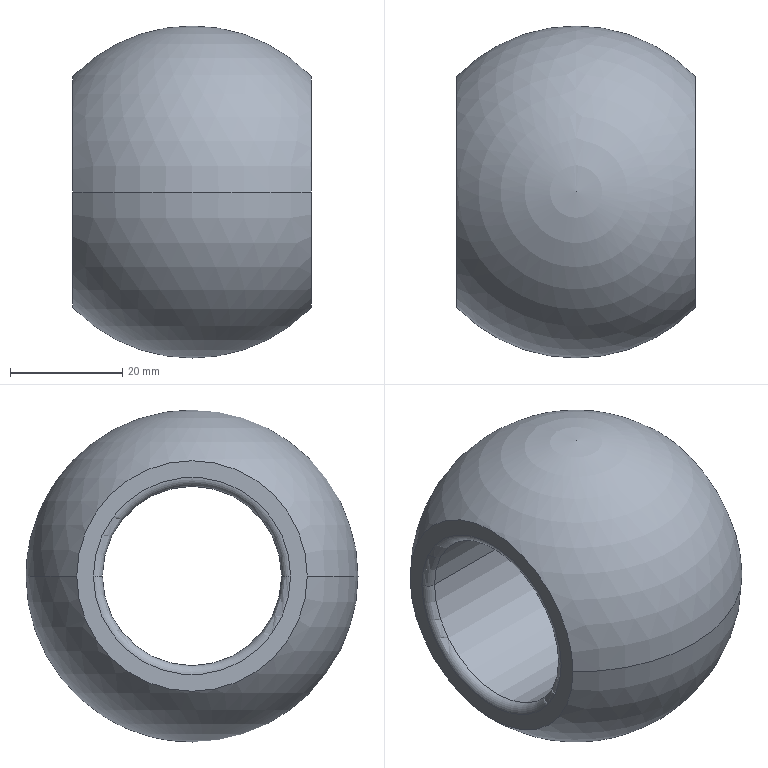Part | STEP file | Large rod end bearing | 1 solid | 10 faces | box 42.667 x 59.28 x 59.28 mm | volume 62997 mm3 | torus 4 | sphere 2 | cylinder 2 | plane 2 | commonest cylinder face diameters 32 x2
STEP:
#1=CARTESIAN_POINT('',(21.333,20.577,261.));
#2=VERTEX_POINT('',#1);
#3=CARTESIAN_POINT('',(21.333,-20.577,261.));
#4=VERTEX_POINT('',#3);
#5=CARTESIAN_POINT('',(21.333,0.,261.));
#6=DIRECTION('',(-1.,0.,0.));
#7=DIRECTION('',(0.,-1.,0.));
#8=AXIS2_PLACEMENT_3D('',#5,#6,#7);
#9=CIRCLE('',#8,20.577);
#10=EDGE_CURVE('',#2,#4,#9,.T.);
#11=ORIENTED_EDGE('',*,*,#10,.T.);
#12=CARTESIAN_POINT('',(-21.333,-20.577,261.));
#13=VERTEX_POINT('',#12);
#14=CARTESIAN_POINT('',(0.,0.,261.));
#15=DIRECTION('',(0.,0.,-1.));
#16=DIRECTION('',(0.,1.,0.));
#17=AXIS2_PLACEMENT_3D('',#14,#15,#16);
#18=CIRCLE('',#17,29.64);
#19=EDGE_CURVE('',#4,#13,#18,.T.);
#20=ORIENTED_EDGE('',*,*,#19,.T.);
#21=CARTESIAN_POINT('',(-21.333,20.577,261.));
#22=VERTEX_POINT('',#21);
#23=CARTESIAN_POINT('',(-21.333,0.,261.));
#24=DIRECTION('',(-1.,0.,0.));
#25=DIRECTION('',(0.,-1.,0.));
#26=AXIS2_PLACEMENT_3D('',#23,#24,#25);
#27=CIRCLE('',#26,20.577);
#28=EDGE_CURVE('',#22,#13,#27,.T.);
#29=ORIENTED_EDGE('',*,*,#28,.F.);
#30=CARTESIAN_POINT('',(0.,0.,261.));
#31=DIRECTION('',(0.,0.,1.));
#32=DIRECTION('',(1.,0.,0.));
#33=AXIS2_PLACEMENT_3D('',#30,#31,#32);
#34=CIRCLE('',#33,29.64);
#35=EDGE_CURVE('',#2,#22,#34,.T.);
#36=ORIENTED_EDGE('',*,*,#35,.F.);
#37=EDGE_LOOP('',(#11,#20,#29,#36));
#38=FACE_OUTER_BOUND('',#37,.T.);
#39=CARTESIAN_POINT('',(0.,0.,261.));
#40=DIRECTION('',(0.,0.,-1.));
#41=DIRECTION('',(0.,1.,0.));
#42=AXIS2_PLACEMENT_3D('',#39,#40,#41);
#43=SPHERICAL_SURFACE('',#42,29.64);
#44=ADVANCED_FACE('',(#38),#43,.T.);
#45=CARTESIAN_POINT('',(-21.333,-17.6,261.));
#46=VERTEX_POINT('',#45);
#47=CARTESIAN_POINT('',(-21.333,17.6,261.));
#48=VERTEX_POINT('',#47);
#49=CARTESIAN_POINT('',(-21.333,0.,261.));
#50=DIRECTION('',(-1.,0.,0.));
#51=DIRECTION('',(0.,-1.,0.));
#52=AXIS2_PLACEMENT_3D('',#49,#50,#51);
#53=CIRCLE('',#52,17.6);
#54=EDGE_CURVE('',#46,#48,#53,.T.);
#55=ORIENTED_EDGE('',*,*,#54,.T.);
#56=CARTESIAN_POINT('',(-19.733,16.,261.));
#57=VERTEX_POINT('',#56);
#58=CARTESIAN_POINT('',(-19.733,17.6,261.));
#59=DIRECTION('',(0.,0.,1.));
#60=DIRECTION('',(0.,-1.,0.));
#61=AXIS2_PLACEMENT_3D('',#58,#59,#60);
#62=CIRCLE('',#61,1.6);
#63=EDGE_CURVE('',#48,#57,#62,.T.);
#64=ORIENTED_EDGE('',*,*,#63,.T.);
#65=CARTESIAN_POINT('',(-19.733,-16.,261.));
#66=VERTEX_POINT('',#65);
#67=CARTESIAN_POINT('',(-19.733,0.,261.));
#68=DIRECTION('',(-1.,0.,0.));
#69=DIRECTION('',(0.,-1.,0.));
#70=AXIS2_PLACEMENT_3D('',#67,#68,#69);
#71=CIRCLE('',#70,16.);
#72=EDGE_CURVE('',#66,#57,#71,.T.);
#73=ORIENTED_EDGE('',*,*,#72,.F.);
#74=CARTESIAN_POINT('',(-19.733,-17.6,261.));
#75=DIRECTION('',(0.,0.,-1.));
#76=DIRECTION('',(-1.,0.,0.));
#77=AXIS2_PLACEMENT_3D('',#74,#75,#76);
#78=CIRCLE('',#77,1.6);
#79=EDGE_CURVE('',#46,#66,#78,.T.);
#80=ORIENTED_EDGE('',*,*,#79,.F.);
#81=EDGE_LOOP('',(#55,#64,#73,#80));
#82=FACE_OUTER_BOUND('',#81,.T.);
#83=CARTESIAN_POINT('',(-19.733,0.,261.));
#84=DIRECTION('',(-1.,0.,0.));
#85=DIRECTION('',(0.,-1.,0.));
#86=AXIS2_PLACEMENT_3D('',#83,#84,#85);
#87=TOROIDAL_SURFACE('',#86,17.6,1.6);
#88=ADVANCED_FACE('',(#82),#87,.T.);
#89=CARTESIAN_POINT('',(19.733,16.,261.));
#90=VERTEX_POINT('',#89);
#91=CARTESIAN_POINT('',(19.733,-16.,261.));
#92=VERTEX_POINT('',#91);
#93=CARTESIAN_POINT('',(19.733,0.,261.));
#94=DIRECTION('',(-1.,0.,0.));
#95=DIRECTION('',(0.,-1.,0.));
#96=AXIS2_PLACEMENT_3D('',#93,#94,#95);
#97=CIRCLE('',#96,16.);
#98=EDGE_CURVE('',#90,#92,#97,.T.);
#99=ORIENTED_EDGE('',*,*,#98,.F.);
#100=CARTESIAN_POINT('',(21.333,16.,261.));
#101=DIRECTION('',(-1.,0.,0.));
#102=VECTOR('',#101,1000.);
#103=LINE('',#100,#102);
#104=EDGE_CURVE('',#90,#57,#103,.T.);
#105=ORIENTED_EDGE('',*,*,#104,.T.);
#106=CARTESIAN_POINT('',(-19.733,0.,261.));
#107=DIRECTION('',(-1.,0.,0.));
#108=DIRECTION('',(0.,-1.,0.));
#109=AXIS2_PLACEMENT_3D('',#106,#107,#108);
#110=CIRCLE('',#109,16.);
#111=EDGE_CURVE('',#57,#66,#110,.T.);
#112=ORIENTED_EDGE('',*,*,#111,.T.);
#113=CARTESIAN_POINT('',(21.333,-16.,261.));
#114=DIRECTION('',(-1.,0.,0.));
#115=VECTOR('',#114,1000.);
#116=LINE('',#113,#115);
#117=EDGE_CURVE('',#92,#66,#116,.T.);
#118=ORIENTED_EDGE('',*,*,#117,.F.);
#119=EDGE_LOOP('',(#99,#105,#112,#118));
#120=FACE_OUTER_BOUND('',#119,.T.);
#121=CARTESIAN_POINT('',(21.333,0.,261.));
#122=DIRECTION('',(-1.,0.,0.));
#123=DIRECTION('',(0.,-1.,0.));
#124=AXIS2_PLACEMENT_3D('',#121,#122,#123);
#125=CYLINDRICAL_SURFACE('',#124,16.);
#126=ADVANCED_FACE('',(#120),#125,.F.);
#127=CARTESIAN_POINT('',(19.733,0.,261.));
#128=DIRECTION('',(-1.,0.,0.));
#129=DIRECTION('',(0.,-1.,0.));
#130=AXIS2_PLACEMENT_3D('',#127,#128,#129);
#131=CIRCLE('',#130,16.);
#132=EDGE_CURVE('',#92,#90,#131,.T.);
#133=ORIENTED_EDGE('',*,*,#132,.T.);
#134=CARTESIAN_POINT('',(21.333,17.6,261.));
#135=VERTEX_POINT('',#134);
#136=CARTESIAN_POINT('',(19.733,17.6,261.));
#137=DIRECTION('',(0.,0.,1.));
#138=DIRECTION('',(0.,-1.,0.));
#139=AXIS2_PLACEMENT_3D('',#136,#137,#138);
#140=CIRCLE('',#139,1.6);
#141=EDGE_CURVE('',#90,#135,#140,.T.);
#142=ORIENTED_EDGE('',*,*,#141,.T.);
#143=CARTESIAN_POINT('',(21.333,-17.6,261.));
#144=VERTEX_POINT('',#143);
#145=CARTESIAN_POINT('',(21.333,0.,261.));
#146=DIRECTION('',(-1.,0.,0.));
#147=DIRECTION('',(0.,-1.,0.));
#148=AXIS2_PLACEMENT_3D('',#145,#146,#147);
#149=CIRCLE('',#148,17.6);
#150=EDGE_CURVE('',#144,#135,#149,.T.);
#151=ORIENTED_EDGE('',*,*,#150,.F.);
#152=CARTESIAN_POINT('',(19.733,-17.6,261.));
#153=DIRECTION('',(0.,0.,-1.));
#154=DIRECTION('',(-1.,0.,0.));
#155=AXIS2_PLACEMENT_3D('',#152,#153,#154);
#156=CIRCLE('',#155,1.6);
#157=EDGE_CURVE('',#92,#144,#156,.T.);
#158=ORIENTED_EDGE('',*,*,#157,.F.);
#159=EDGE_LOOP('',(#133,#142,#151,#158));
#160=FACE_OUTER_BOUND('',#159,.T.);
#161=CARTESIAN_POINT('',(19.733,0.,261.));
#162=DIRECTION('',(-1.,0.,0.));
#163=DIRECTION('',(0.,-1.,0.));
#164=AXIS2_PLACEMENT_3D('',#161,#162,#163);
#165=TOROIDAL_SURFACE('',#164,17.6,1.6);
#166=ADVANCED_FACE('',(#160),#165,.T.);
#167=ORIENTED_EDGE('',*,*,#141,.F.);
#168=ORIENTED_EDGE('',*,*,#98,.T.);
#169=ORIENTED_EDGE('',*,*,#157,.T.);
#170=CARTESIAN_POINT('',(21.333,0.,261.));
#171=DIRECTION('',(-1.,0.,0.));
#172=DIRECTION('',(0.,-1.,0.));
#173=AXIS2_PLACEMENT_3D('',#170,#171,#172);
#174=CIRCLE('',#173,17.6);
#175=EDGE_CURVE('',#135,#144,#174,.T.);
#176=ORIENTED_EDGE('',*,*,#175,.F.);
#177=EDGE_LOOP('',(#167,#168,#169,#176));
#178=FACE_OUTER_BOUND('',#177,.T.);
#179=CARTESIAN_POINT('',(19.733,0.,261.));
#180=DIRECTION('',(-1.,0.,0.));
#181=DIRECTION('',(0.,-1.,0.));
#182=AXIS2_PLACEMENT_3D('',#179,#180,#181);
#183=TOROIDAL_SURFACE('',#182,17.6,1.6);
#184=ADVANCED_FACE('',(#178),#183,.T.);
#185=ORIENTED_EDGE('',*,*,#104,.F.);
#186=ORIENTED_EDGE('',*,*,#132,.F.);
#187=ORIENTED_EDGE('',*,*,#117,.T.);
#188=ORIENTED_EDGE('',*,*,#72,.T.);
#189=EDGE_LOOP('',(#185,#186,#187,#188));
#190=FACE_OUTER_BOUND('',#189,.T.);
#191=CARTESIAN_POINT('',(21.333,0.,261.));
#192=DIRECTION('',(-1.,0.,0.));
#193=DIRECTION('',(0.,-1.,0.));
#194=AXIS2_PLACEMENT_3D('',#191,#192,#193);
#195=CYLINDRICAL_SURFACE('',#194,16.);
#196=ADVANCED_FACE('',(#190),#195,.F.);
#197=ORIENTED_EDGE('',*,*,#63,.F.);
#198=CARTESIAN_POINT('',(-21.333,0.,261.));
#199=DIRECTION('',(-1.,0.,0.));
#200=DIRECTION('',(0.,-1.,0.));
#201=AXIS2_PLACEMENT_3D('',#198,#199,#200);
#202=CIRCLE('',#201,17.6);
#203=EDGE_CURVE('',#48,#46,#202,.T.);
#204=ORIENTED_EDGE('',*,*,#203,.T.);
#205=ORIENTED_EDGE('',*,*,#79,.T.);
#206=ORIENTED_EDGE('',*,*,#111,.F.);
#207=EDGE_LOOP('',(#197,#204,#205,#206));
#208=FACE_OUTER_BOUND('',#207,.T.);
#209=CARTESIAN_POINT('',(-19.733,0.,261.));
#210=DIRECTION('',(-1.,0.,0.));
#211=DIRECTION('',(0.,-1.,0.));
#212=AXIS2_PLACEMENT_3D('',#209,#210,#211);
#213=TOROIDAL_SURFACE('',#212,17.6,1.6);
#214=ADVANCED_FACE('',(#208),#213,.T.);
#215=ORIENTED_EDGE('',*,*,#28,.T.);
#216=CARTESIAN_POINT('',(-21.333,0.,261.));
#217=DIRECTION('',(-1.,0.,0.));
#218=DIRECTION('',(0.,-1.,0.));
#219=AXIS2_PLACEMENT_3D('',#216,#217,#218);
#220=CIRCLE('',#219,20.577);
#221=EDGE_CURVE('',#13,#22,#220,.T.);
#222=ORIENTED_EDGE('',*,*,#221,.T.);
#223=EDGE_LOOP('',(#215,#222));
#224=FACE_OUTER_BOUND('',#223,.T.);
#225=ORIENTED_EDGE('',*,*,#54,.F.);
#226=ORIENTED_EDGE('',*,*,#203,.F.);
#227=EDGE_LOOP('',(#225,#226));
#228=FACE_BOUND('',#227,.T.);
#229=CARTESIAN_POINT('',(-21.333,17.6,261.));
#230=DIRECTION('',(-1.,0.,0.));
#231=DIRECTION('',(0.,-1.,0.));
#232=AXIS2_PLACEMENT_3D('',#229,#230,#231);
#233=PLANE('',#232);
#234=ADVANCED_FACE('',(#224,#228),#233,.T.);
#235=ORIENTED_EDGE('',*,*,#19,.F.);
#236=CARTESIAN_POINT('',(21.333,0.,261.));
#237=DIRECTION('',(-1.,0.,0.));
#238=DIRECTION('',(0.,-1.,0.));
#239=AXIS2_PLACEMENT_3D('',#236,#237,#238);
#240=CIRCLE('',#239,20.577);
#241=EDGE_CURVE('',#4,#2,#240,.T.);
#242=ORIENTED_EDGE('',*,*,#241,.T.);
#243=ORIENTED_EDGE('',*,*,#35,.T.);
#244=ORIENTED_EDGE('',*,*,#221,.F.);
#245=EDGE_LOOP('',(#235,#242,#243,#244));
#246=FACE_OUTER_BOUND('',#245,.T.);
#247=CARTESIAN_POINT('',(0.,0.,261.));
#248=DIRECTION('',(0.,0.,-1.));
#249=DIRECTION('',(0.,1.,0.));
#250=AXIS2_PLACEMENT_3D('',#247,#248,#249);
#251=SPHERICAL_SURFACE('',#250,29.64);
#252=ADVANCED_FACE('',(#246),#251,.T.);
#253=ORIENTED_EDGE('',*,*,#150,.T.);
#254=ORIENTED_EDGE('',*,*,#175,.T.);
#255=EDGE_LOOP('',(#253,#254));
#256=FACE_BOUND('',#255,.T.);
#257=ORIENTED_EDGE('',*,*,#10,.F.);
#258=ORIENTED_EDGE('',*,*,#241,.F.);
#259=EDGE_LOOP('',(#257,#258));
#260=FACE_OUTER_BOUND('',#259,.T.);
#261=CARTESIAN_POINT('',(21.333,20.577,261.));
#262=DIRECTION('',(1.,0.,0.));
#263=DIRECTION('',(0.,1.,0.));
#264=AXIS2_PLACEMENT_3D('',#261,#262,#263);
#265=PLANE('',#264);
#266=ADVANCED_FACE('',(#256,#260),#265,.T.);
#267=CLOSED_SHELL('',(#44,#88,#126,#166,#184,#196,#214,#234,#252,#266));
#268=MANIFOLD_SOLID_BREP('',#267);
#269=CARTESIAN_POINT('',(0.,0.,0.));
#270=DIRECTION('',(0.,0.,1.));
#271=DIRECTION('',(1.,0.,0.));
#272=AXIS2_PLACEMENT_3D('',#269,#270,#271);
#273=(LENGTH_UNIT()NAMED_UNIT(*)SI_UNIT(.MILLI.,.METRE.));
#274=UNCERTAINTY_MEASURE_WITH_UNIT(LENGTH_MEASURE(0.00001),#273,'','');
#275=(NAMED_UNIT(*)PLANE_ANGLE_UNIT()SI_UNIT($,.RADIAN.));
#276=(NAMED_UNIT(*)SI_UNIT($,.STERADIAN.)SOLID_ANGLE_UNIT());
#277=(GEOMETRIC_REPRESENTATION_CONTEXT(3)GLOBAL_UNCERTAINTY_ASSIGNED_CONTEXT((#274))GLOBAL_UNIT_ASSIGNED_CONTEXT((#273,#275,#276))REPRESENTATION_CONTEXT('',''));
#278=ADVANCED_BREP_SHAPE_REPRESENTATION('',(#268,#272),#277);